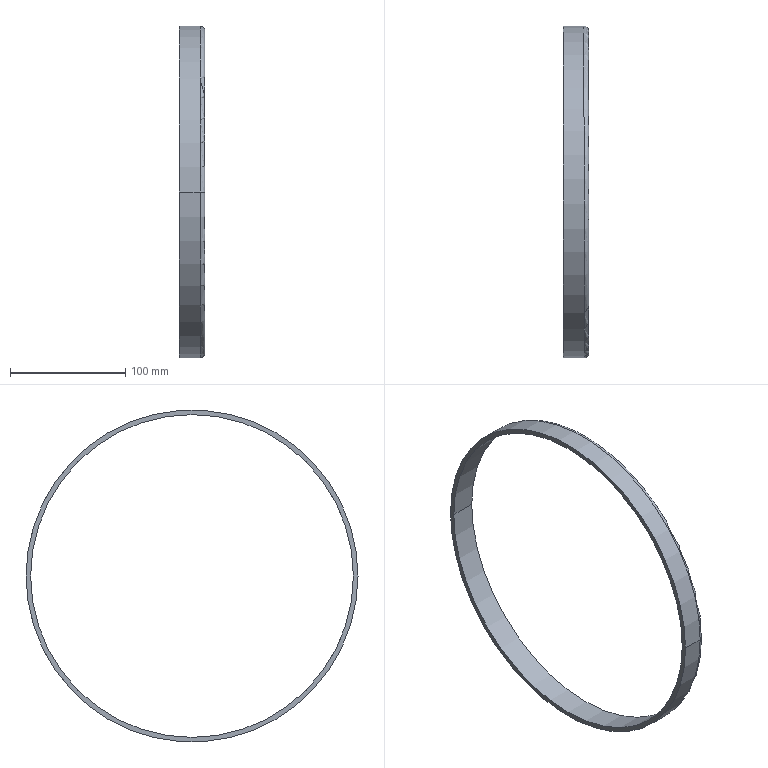Part | SolidWorks | features BaseBody 1 | 1 solid | 7 faces | box 22.273 x 288.017 x 288 mm | volume 75427 mm3 | cylinder 4 | torus 2 | plane 1 | commonest cylinder face diameters 280 x2 288 x2
STEP:
#1=CARTESIAN_POINT('',(294.744,609.919,106.919));
#2=VERTEX_POINT('',#1);
#3=CARTESIAN_POINT('',(295.021,321.919,106.919));
#4=VERTEX_POINT('',#3);
#5=CARTESIAN_POINT('',(294.883,465.919,106.919));
#6=DIRECTION('',(-1.,-0.0009599,0.));
#7=DIRECTION('',(-0.0009599,1.,0.));
#8=AXIS2_PLACEMENT_3D('',#5,#6,#7);
#9=CIRCLE('',#8,144.);
#10=EDGE_CURVE('',#2,#4,#9,.T.);
#11=ORIENTED_EDGE('',*,*,#10,.F.);
#12=CARTESIAN_POINT('',(312.744,609.936,106.919));
#13=VERTEX_POINT('',#12);
#14=CARTESIAN_POINT('',(294.744,609.919,106.919));
#15=DIRECTION('',(1.,0.0009599,0.));
#16=VECTOR('',#15,1000.);
#17=LINE('',#14,#16);
#18=EDGE_CURVE('',#2,#13,#17,.T.);
#19=ORIENTED_EDGE('',*,*,#18,.T.);
#20=CARTESIAN_POINT('',(313.021,321.936,106.919));
#21=VERTEX_POINT('',#20);
#22=CARTESIAN_POINT('',(312.883,465.936,106.919));
#23=DIRECTION('',(1.,0.0009599,0.));
#24=DIRECTION('',(0.0009599,-1.,0.));
#25=AXIS2_PLACEMENT_3D('',#22,#23,#24);
#26=CIRCLE('',#25,144.);
#27=EDGE_CURVE('',#21,#13,#26,.T.);
#28=ORIENTED_EDGE('',*,*,#27,.F.);
#29=CARTESIAN_POINT('',(295.021,321.919,106.919));
#30=DIRECTION('',(1.,0.0009599,0.));
#31=VECTOR('',#30,1000.);
#32=LINE('',#29,#31);
#33=EDGE_CURVE('',#4,#21,#32,.T.);
#34=ORIENTED_EDGE('',*,*,#33,.F.);
#35=EDGE_LOOP('',(#11,#19,#28,#34));
#36=FACE_OUTER_BOUND('',#35,.T.);
#37=CARTESIAN_POINT('',(294.883,465.919,106.919));
#38=DIRECTION('',(1.,0.0009599,0.));
#39=DIRECTION('',(0.0009599,-1.,0.));
#40=AXIS2_PLACEMENT_3D('',#37,#38,#39);
#41=CYLINDRICAL_SURFACE('',#40,144.);
#42=ADVANCED_FACE('',(#36),#41,.T.);
#43=ORIENTED_EDGE('',*,*,#27,.T.);
#44=CARTESIAN_POINT('',(316.748,605.94,106.919));
#45=VERTEX_POINT('',#44);
#46=CARTESIAN_POINT('',(312.748,605.936,106.919));
#47=DIRECTION('',(0.,0.,-1.));
#48=DIRECTION('',(0.,1.,0.));
#49=AXIS2_PLACEMENT_3D('',#46,#47,#48);
#50=CIRCLE('',#49,4.);
#51=EDGE_CURVE('',#13,#45,#50,.T.);
#52=ORIENTED_EDGE('',*,*,#51,.T.);
#53=CARTESIAN_POINT('',(317.017,325.94,106.919));
#54=VERTEX_POINT('',#53);
#55=CARTESIAN_POINT('',(316.883,465.94,106.919));
#56=DIRECTION('',(-1.,-0.0009599,0.));
#57=DIRECTION('',(-0.0009599,1.,0.));
#58=AXIS2_PLACEMENT_3D('',#55,#56,#57);
#59=CIRCLE('',#58,140.);
#60=EDGE_CURVE('',#45,#54,#59,.T.);
#61=ORIENTED_EDGE('',*,*,#60,.T.);
#62=CARTESIAN_POINT('',(313.017,325.936,106.919));
#63=DIRECTION('',(0.,0.,1.));
#64=DIRECTION('',(1.,0.,0.));
#65=AXIS2_PLACEMENT_3D('',#62,#63,#64);
#66=CIRCLE('',#65,4.);
#67=EDGE_CURVE('',#21,#54,#66,.T.);
#68=ORIENTED_EDGE('',*,*,#67,.F.);
#69=EDGE_LOOP('',(#43,#52,#61,#68));
#70=FACE_OUTER_BOUND('',#69,.T.);
#71=CARTESIAN_POINT('',(312.883,465.936,106.919));
#72=DIRECTION('',(1.,0.0009599,0.));
#73=DIRECTION('',(0.0009599,-1.,0.));
#74=AXIS2_PLACEMENT_3D('',#71,#72,#73);
#75=TOROIDAL_SURFACE('',#74,140.,4.);
#76=ADVANCED_FACE('',(#70),#75,.T.);
#77=CARTESIAN_POINT('',(294.748,605.919,106.919));
#78=VERTEX_POINT('',#77);
#79=CARTESIAN_POINT('',(295.017,325.919,106.919));
#80=VERTEX_POINT('',#79);
#81=CARTESIAN_POINT('',(294.883,465.919,106.919));
#82=DIRECTION('',(1.,0.0009599,0.));
#83=DIRECTION('',(-0.0009599,1.,0.));
#84=AXIS2_PLACEMENT_3D('',#81,#82,#83);
#85=CIRCLE('',#84,140.);
#86=EDGE_CURVE('',#78,#80,#85,.T.);
#87=ORIENTED_EDGE('',*,*,#86,.F.);
#88=CARTESIAN_POINT('',(294.748,605.919,106.919));
#89=DIRECTION('',(1.,0.0009599,0.));
#90=VECTOR('',#89,1000.);
#91=LINE('',#88,#90);
#92=EDGE_CURVE('',#78,#45,#91,.T.);
#93=ORIENTED_EDGE('',*,*,#92,.T.);
#94=CARTESIAN_POINT('',(316.883,465.94,106.919));
#95=DIRECTION('',(-1.,-0.0009599,0.));
#96=DIRECTION('',(-0.0009599,1.,0.));
#97=AXIS2_PLACEMENT_3D('',#94,#95,#96);
#98=CIRCLE('',#97,140.);
#99=EDGE_CURVE('',#54,#45,#98,.T.);
#100=ORIENTED_EDGE('',*,*,#99,.F.);
#101=CARTESIAN_POINT('',(295.017,325.919,106.919));
#102=DIRECTION('',(1.,0.0009599,0.));
#103=VECTOR('',#102,1000.);
#104=LINE('',#101,#103);
#105=EDGE_CURVE('',#80,#54,#104,.T.);
#106=ORIENTED_EDGE('',*,*,#105,.F.);
#107=EDGE_LOOP('',(#87,#93,#100,#106));
#108=FACE_OUTER_BOUND('',#107,.T.);
#109=CARTESIAN_POINT('',(294.883,465.919,106.919));
#110=DIRECTION('',(1.,0.0009599,0.));
#111=DIRECTION('',(0.0009599,-1.,0.));
#112=AXIS2_PLACEMENT_3D('',#109,#110,#111);
#113=CYLINDRICAL_SURFACE('',#112,140.);
#114=ADVANCED_FACE('',(#108),#113,.F.);
#115=ORIENTED_EDGE('',*,*,#92,.F.);
#116=CARTESIAN_POINT('',(294.883,465.919,106.919));
#117=DIRECTION('',(1.,0.0009599,0.));
#118=DIRECTION('',(-0.0009599,1.,0.));
#119=AXIS2_PLACEMENT_3D('',#116,#117,#118);
#120=CIRCLE('',#119,140.);
#121=EDGE_CURVE('',#80,#78,#120,.T.);
#122=ORIENTED_EDGE('',*,*,#121,.F.);
#123=ORIENTED_EDGE('',*,*,#105,.T.);
#124=ORIENTED_EDGE('',*,*,#60,.F.);
#125=EDGE_LOOP('',(#115,#122,#123,#124));
#126=FACE_OUTER_BOUND('',#125,.T.);
#127=CARTESIAN_POINT('',(294.883,465.919,106.919));
#128=DIRECTION('',(1.,0.0009599,0.));
#129=DIRECTION('',(0.0009599,-1.,0.));
#130=AXIS2_PLACEMENT_3D('',#127,#128,#129);
#131=CYLINDRICAL_SURFACE('',#130,140.);
#132=ADVANCED_FACE('',(#126),#131,.F.);
#133=ORIENTED_EDGE('',*,*,#121,.T.);
#134=ORIENTED_EDGE('',*,*,#86,.T.);
#135=EDGE_LOOP('',(#133,#134));
#136=FACE_BOUND('',#135,.T.);
#137=CARTESIAN_POINT('',(294.883,465.919,106.919));
#138=DIRECTION('',(-1.,-0.0009599,0.));
#139=DIRECTION('',(-0.0009599,1.,0.));
#140=AXIS2_PLACEMENT_3D('',#137,#138,#139);
#141=CIRCLE('',#140,144.);
#142=EDGE_CURVE('',#4,#2,#141,.T.);
#143=ORIENTED_EDGE('',*,*,#142,.T.);
#144=ORIENTED_EDGE('',*,*,#10,.T.);
#145=EDGE_LOOP('',(#143,#144));
#146=FACE_OUTER_BOUND('',#145,.T.);
#147=CARTESIAN_POINT('',(294.883,465.919,106.919));
#148=DIRECTION('',(1.,0.0009599,0.));
#149=DIRECTION('',(0.,0.,-1.));
#150=AXIS2_PLACEMENT_3D('',#147,#148,#149);
#151=PLANE('',#150);
#152=ADVANCED_FACE('',(#136,#146),#151,.F.);
#153=ORIENTED_EDGE('',*,*,#51,.F.);
#154=CARTESIAN_POINT('',(312.883,465.936,106.919));
#155=DIRECTION('',(1.,0.0009599,0.));
#156=DIRECTION('',(0.0009599,-1.,0.));
#157=AXIS2_PLACEMENT_3D('',#154,#155,#156);
#158=CIRCLE('',#157,144.);
#159=EDGE_CURVE('',#13,#21,#158,.T.);
#160=ORIENTED_EDGE('',*,*,#159,.T.);
#161=ORIENTED_EDGE('',*,*,#67,.T.);
#162=ORIENTED_EDGE('',*,*,#99,.T.);
#163=EDGE_LOOP('',(#153,#160,#161,#162));
#164=FACE_OUTER_BOUND('',#163,.T.);
#165=CARTESIAN_POINT('',(312.883,465.936,106.919));
#166=DIRECTION('',(1.,0.0009599,0.));
#167=DIRECTION('',(0.0009599,-1.,0.));
#168=AXIS2_PLACEMENT_3D('',#165,#166,#167);
#169=TOROIDAL_SURFACE('',#168,140.,4.);
#170=ADVANCED_FACE('',(#164),#169,.T.);
#171=ORIENTED_EDGE('',*,*,#18,.F.);
#172=ORIENTED_EDGE('',*,*,#142,.F.);
#173=ORIENTED_EDGE('',*,*,#33,.T.);
#174=ORIENTED_EDGE('',*,*,#159,.F.);
#175=EDGE_LOOP('',(#171,#172,#173,#174));
#176=FACE_OUTER_BOUND('',#175,.T.);
#177=CARTESIAN_POINT('',(294.883,465.919,106.919));
#178=DIRECTION('',(1.,0.0009599,0.));
#179=DIRECTION('',(0.0009599,-1.,0.));
#180=AXIS2_PLACEMENT_3D('',#177,#178,#179);
#181=CYLINDRICAL_SURFACE('',#180,144.);
#182=ADVANCED_FACE('',(#176),#181,.T.);
#183=CLOSED_SHELL('',(#42,#76,#114,#132,#152,#170,#182));
#184=MANIFOLD_SOLID_BREP('',#183);
#185=CARTESIAN_POINT('',(0.,0.,0.));
#186=DIRECTION('',(0.,0.,1.));
#187=DIRECTION('',(1.,0.,0.));
#188=AXIS2_PLACEMENT_3D('',#185,#186,#187);
#189=(LENGTH_UNIT()NAMED_UNIT(*)SI_UNIT(.MILLI.,.METRE.));
#190=UNCERTAINTY_MEASURE_WITH_UNIT(LENGTH_MEASURE(0.00001),#189,'','');
#191=(NAMED_UNIT(*)PLANE_ANGLE_UNIT()SI_UNIT($,.RADIAN.));
#192=(NAMED_UNIT(*)SI_UNIT($,.STERADIAN.)SOLID_ANGLE_UNIT());
#193=(GEOMETRIC_REPRESENTATION_CONTEXT(3)GLOBAL_UNCERTAINTY_ASSIGNED_CONTEXT((#190))GLOBAL_UNIT_ASSIGNED_CONTEXT((#189,#191,#192))REPRESENTATION_CONTEXT('',''));
#194=ADVANCED_BREP_SHAPE_REPRESENTATION('',(#184,#188),#193);